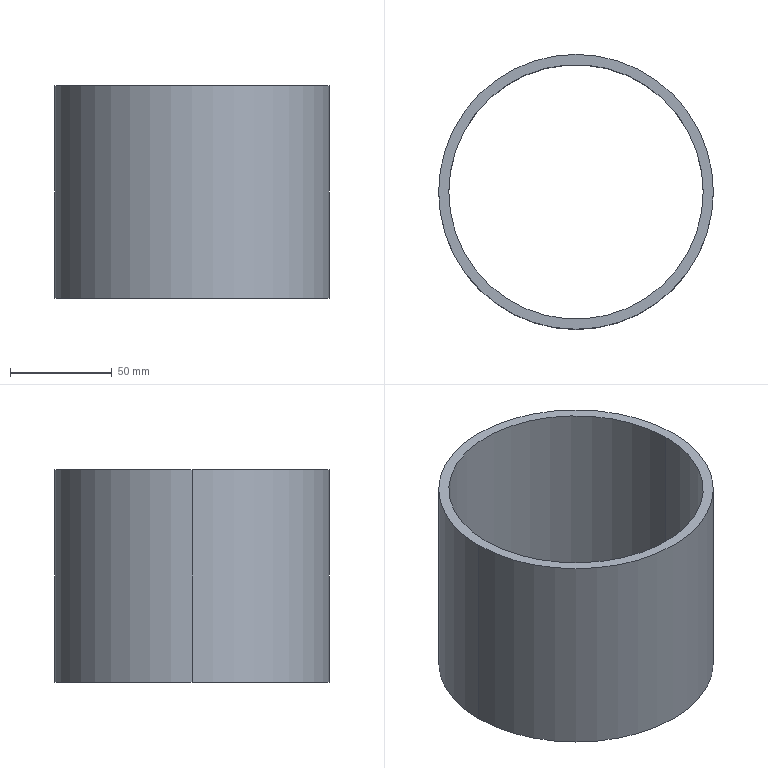Part | SolidWorks | features BaseBody 1 | 1 solid | 6 faces | box 135 x 135 x 104.3 mm | volume 212984 mm3 | cylinder 4 | plane 2 | commonest cylinder face diameters 125 x2 135 x2
STEP:
#1=CARTESIAN_POINT('',(-144.401,35.943,104.3));
#2=VERTEX_POINT('',#1);
#3=CARTESIAN_POINT('',(-9.401,35.943,104.3));
#4=VERTEX_POINT('',#3);
#5=CARTESIAN_POINT('',(-76.901,35.943,104.3));
#6=DIRECTION('',(0.,0.,-1.));
#7=DIRECTION('',(-1.,0.,0.));
#8=AXIS2_PLACEMENT_3D('',#5,#6,#7);
#9=CIRCLE('',#8,67.5);
#10=EDGE_CURVE('',#2,#4,#9,.T.);
#11=ORIENTED_EDGE('',*,*,#10,.T.);
#12=CARTESIAN_POINT('',(-9.401,35.943,0.));
#13=VERTEX_POINT('',#12);
#14=CARTESIAN_POINT('',(-9.401,35.943,104.3));
#15=DIRECTION('',(0.,0.,-1.));
#16=VECTOR('',#15,1000.);
#17=LINE('',#14,#16);
#18=EDGE_CURVE('',#4,#13,#17,.T.);
#19=ORIENTED_EDGE('',*,*,#18,.T.);
#20=CARTESIAN_POINT('',(-144.401,35.943,0.));
#21=VERTEX_POINT('',#20);
#22=CARTESIAN_POINT('',(-76.901,35.943,0.));
#23=DIRECTION('',(0.,0.,1.));
#24=DIRECTION('',(-1.,0.,0.));
#25=AXIS2_PLACEMENT_3D('',#22,#23,#24);
#26=CIRCLE('',#25,67.5);
#27=EDGE_CURVE('',#13,#21,#26,.T.);
#28=ORIENTED_EDGE('',*,*,#27,.T.);
#29=CARTESIAN_POINT('',(-144.401,35.943,104.3));
#30=DIRECTION('',(0.,0.,-1.));
#31=VECTOR('',#30,1000.);
#32=LINE('',#29,#31);
#33=EDGE_CURVE('',#2,#21,#32,.T.);
#34=ORIENTED_EDGE('',*,*,#33,.F.);
#35=EDGE_LOOP('',(#11,#19,#28,#34));
#36=FACE_OUTER_BOUND('',#35,.T.);
#37=CARTESIAN_POINT('',(-76.901,35.943,104.3));
#38=DIRECTION('',(0.,0.,-1.));
#39=DIRECTION('',(-1.,0.,0.));
#40=AXIS2_PLACEMENT_3D('',#37,#38,#39);
#41=CYLINDRICAL_SURFACE('',#40,67.5);
#42=ADVANCED_FACE('',(#36),#41,.T.);
#43=CARTESIAN_POINT('',(-14.401,35.943,104.3));
#44=VERTEX_POINT('',#43);
#45=CARTESIAN_POINT('',(-139.401,35.943,104.3));
#46=VERTEX_POINT('',#45);
#47=CARTESIAN_POINT('',(-76.901,35.943,104.3));
#48=DIRECTION('',(0.,0.,-1.));
#49=DIRECTION('',(-1.,0.,0.));
#50=AXIS2_PLACEMENT_3D('',#47,#48,#49);
#51=CIRCLE('',#50,62.5);
#52=EDGE_CURVE('',#44,#46,#51,.T.);
#53=ORIENTED_EDGE('',*,*,#52,.F.);
#54=CARTESIAN_POINT('',(-14.401,35.943,0.));
#55=VERTEX_POINT('',#54);
#56=CARTESIAN_POINT('',(-14.401,35.943,104.3));
#57=DIRECTION('',(0.,0.,-1.));
#58=VECTOR('',#57,1000.);
#59=LINE('',#56,#58);
#60=EDGE_CURVE('',#44,#55,#59,.T.);
#61=ORIENTED_EDGE('',*,*,#60,.T.);
#62=CARTESIAN_POINT('',(-139.401,35.943,0.));
#63=VERTEX_POINT('',#62);
#64=CARTESIAN_POINT('',(-76.901,35.943,0.));
#65=DIRECTION('',(0.,0.,-1.));
#66=DIRECTION('',(-1.,0.,0.));
#67=AXIS2_PLACEMENT_3D('',#64,#65,#66);
#68=CIRCLE('',#67,62.5);
#69=EDGE_CURVE('',#55,#63,#68,.T.);
#70=ORIENTED_EDGE('',*,*,#69,.T.);
#71=CARTESIAN_POINT('',(-139.401,35.943,104.3));
#72=DIRECTION('',(0.,0.,-1.));
#73=VECTOR('',#72,1000.);
#74=LINE('',#71,#73);
#75=EDGE_CURVE('',#46,#63,#74,.T.);
#76=ORIENTED_EDGE('',*,*,#75,.F.);
#77=EDGE_LOOP('',(#53,#61,#70,#76));
#78=FACE_OUTER_BOUND('',#77,.T.);
#79=CARTESIAN_POINT('',(-76.901,35.943,104.3));
#80=DIRECTION('',(0.,0.,-1.));
#81=DIRECTION('',(-1.,0.,0.));
#82=AXIS2_PLACEMENT_3D('',#79,#80,#81);
#83=CYLINDRICAL_SURFACE('',#82,62.5);
#84=ADVANCED_FACE('',(#78),#83,.F.);
#85=ORIENTED_EDGE('',*,*,#18,.F.);
#86=CARTESIAN_POINT('',(-76.901,35.943,104.3));
#87=DIRECTION('',(0.,0.,-1.));
#88=DIRECTION('',(-1.,0.,0.));
#89=AXIS2_PLACEMENT_3D('',#86,#87,#88);
#90=CIRCLE('',#89,67.5);
#91=EDGE_CURVE('',#4,#2,#90,.T.);
#92=ORIENTED_EDGE('',*,*,#91,.T.);
#93=ORIENTED_EDGE('',*,*,#33,.T.);
#94=CARTESIAN_POINT('',(-76.901,35.943,0.));
#95=DIRECTION('',(0.,0.,1.));
#96=DIRECTION('',(-1.,0.,0.));
#97=AXIS2_PLACEMENT_3D('',#94,#95,#96);
#98=CIRCLE('',#97,67.5);
#99=EDGE_CURVE('',#21,#13,#98,.T.);
#100=ORIENTED_EDGE('',*,*,#99,.T.);
#101=EDGE_LOOP('',(#85,#92,#93,#100));
#102=FACE_OUTER_BOUND('',#101,.T.);
#103=CARTESIAN_POINT('',(-76.901,35.943,104.3));
#104=DIRECTION('',(0.,0.,-1.));
#105=DIRECTION('',(-1.,0.,0.));
#106=AXIS2_PLACEMENT_3D('',#103,#104,#105);
#107=CYLINDRICAL_SURFACE('',#106,67.5);
#108=ADVANCED_FACE('',(#102),#107,.T.);
#109=CARTESIAN_POINT('',(-76.901,35.943,0.));
#110=DIRECTION('',(0.,0.,-1.));
#111=DIRECTION('',(-1.,0.,0.));
#112=AXIS2_PLACEMENT_3D('',#109,#110,#111);
#113=CIRCLE('',#112,62.5);
#114=EDGE_CURVE('',#63,#55,#113,.T.);
#115=ORIENTED_EDGE('',*,*,#114,.F.);
#116=ORIENTED_EDGE('',*,*,#69,.F.);
#117=EDGE_LOOP('',(#115,#116));
#118=FACE_BOUND('',#117,.T.);
#119=ORIENTED_EDGE('',*,*,#99,.F.);
#120=ORIENTED_EDGE('',*,*,#27,.F.);
#121=EDGE_LOOP('',(#119,#120));
#122=FACE_OUTER_BOUND('',#121,.T.);
#123=CARTESIAN_POINT('',(-76.901,35.943,0.));
#124=DIRECTION('',(0.,0.,1.));
#125=DIRECTION('',(1.,0.,0.));
#126=AXIS2_PLACEMENT_3D('',#123,#124,#125);
#127=PLANE('',#126);
#128=ADVANCED_FACE('',(#118,#122),#127,.F.);
#129=CARTESIAN_POINT('',(-76.901,35.943,104.3));
#130=DIRECTION('',(0.,0.,-1.));
#131=DIRECTION('',(-1.,0.,0.));
#132=AXIS2_PLACEMENT_3D('',#129,#130,#131);
#133=CIRCLE('',#132,62.5);
#134=EDGE_CURVE('',#46,#44,#133,.T.);
#135=ORIENTED_EDGE('',*,*,#134,.T.);
#136=ORIENTED_EDGE('',*,*,#52,.T.);
#137=EDGE_LOOP('',(#135,#136));
#138=FACE_BOUND('',#137,.T.);
#139=ORIENTED_EDGE('',*,*,#10,.F.);
#140=ORIENTED_EDGE('',*,*,#91,.F.);
#141=EDGE_LOOP('',(#139,#140));
#142=FACE_OUTER_BOUND('',#141,.T.);
#143=CARTESIAN_POINT('',(-76.901,35.943,104.3));
#144=DIRECTION('',(0.,0.,1.));
#145=DIRECTION('',(1.,0.,0.));
#146=AXIS2_PLACEMENT_3D('',#143,#144,#145);
#147=PLANE('',#146);
#148=ADVANCED_FACE('',(#138,#142),#147,.T.);
#149=ORIENTED_EDGE('',*,*,#60,.F.);
#150=ORIENTED_EDGE('',*,*,#134,.F.);
#151=ORIENTED_EDGE('',*,*,#75,.T.);
#152=ORIENTED_EDGE('',*,*,#114,.T.);
#153=EDGE_LOOP('',(#149,#150,#151,#152));
#154=FACE_OUTER_BOUND('',#153,.T.);
#155=CARTESIAN_POINT('',(-76.901,35.943,104.3));
#156=DIRECTION('',(0.,0.,-1.));
#157=DIRECTION('',(-1.,0.,0.));
#158=AXIS2_PLACEMENT_3D('',#155,#156,#157);
#159=CYLINDRICAL_SURFACE('',#158,62.5);
#160=ADVANCED_FACE('',(#154),#159,.F.);
#161=CLOSED_SHELL('',(#42,#84,#108,#128,#148,#160));
#162=MANIFOLD_SOLID_BREP('',#161);
#163=CARTESIAN_POINT('',(0.,0.,0.));
#164=DIRECTION('',(0.,0.,1.));
#165=DIRECTION('',(1.,0.,0.));
#166=AXIS2_PLACEMENT_3D('',#163,#164,#165);
#167=(LENGTH_UNIT()NAMED_UNIT(*)SI_UNIT(.MILLI.,.METRE.));
#168=UNCERTAINTY_MEASURE_WITH_UNIT(LENGTH_MEASURE(0.00001),#167,'','');
#169=(NAMED_UNIT(*)PLANE_ANGLE_UNIT()SI_UNIT($,.RADIAN.));
#170=(NAMED_UNIT(*)SI_UNIT($,.STERADIAN.)SOLID_ANGLE_UNIT());
#171=(GEOMETRIC_REPRESENTATION_CONTEXT(3)GLOBAL_UNCERTAINTY_ASSIGNED_CONTEXT((#168))GLOBAL_UNIT_ASSIGNED_CONTEXT((#167,#169,#170))REPRESENTATION_CONTEXT('',''));
#172=ADVANCED_BREP_SHAPE_REPRESENTATION('',(#162,#166),#171);